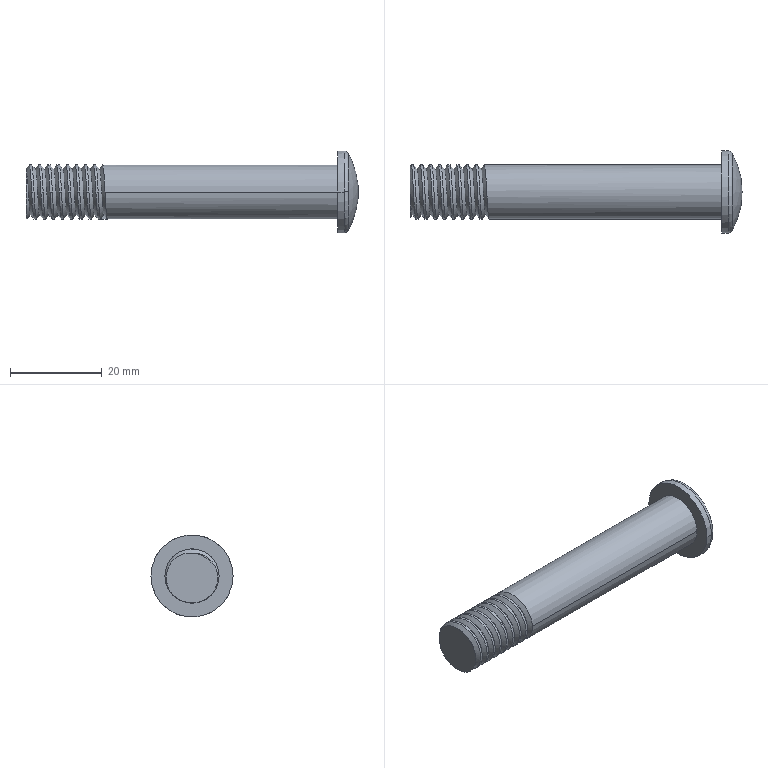Part | NX | features solid 2 | 1 solid | 32 faces | box 72.5 x 17.92 x 17.92 mm | volume 8059 mm3 | cylinder 20 | spline 6 | plane 3 | torus 2 | sphere 1 | commonest cylinder face diameters 11.8 x18 17.92 x2